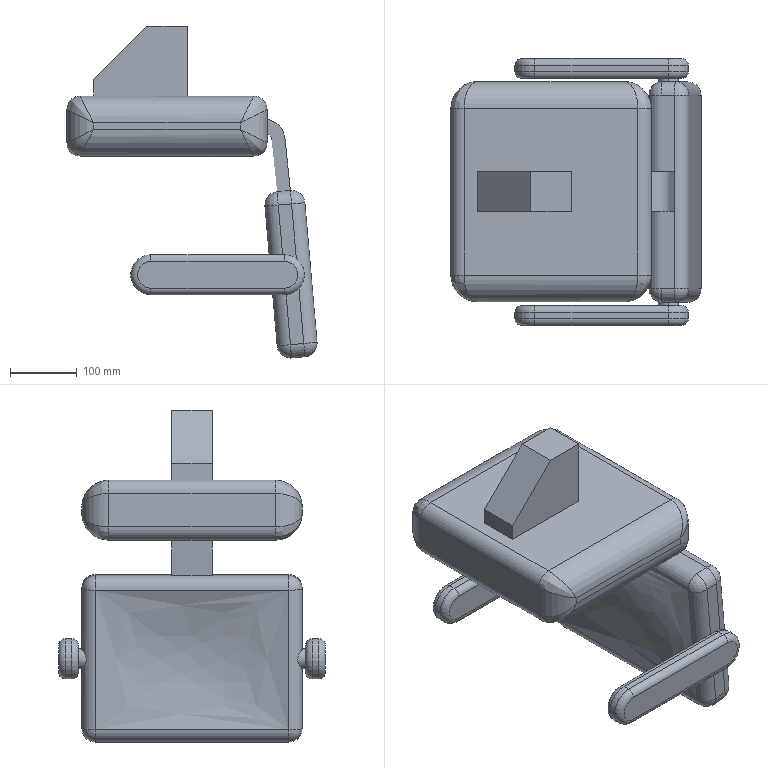Part | SolidWorks | 1 solid | 100 faces | box 374.894 x 400 x 497.382 mm | volume 13317913 mm3 | cylinder 43 | plane 29 | sphere 10 | spline 10 | torus 8 | commonest cylinder face diameters 40 x17 20 x8 80 x8 30 x4 60 x4 25.645 x1